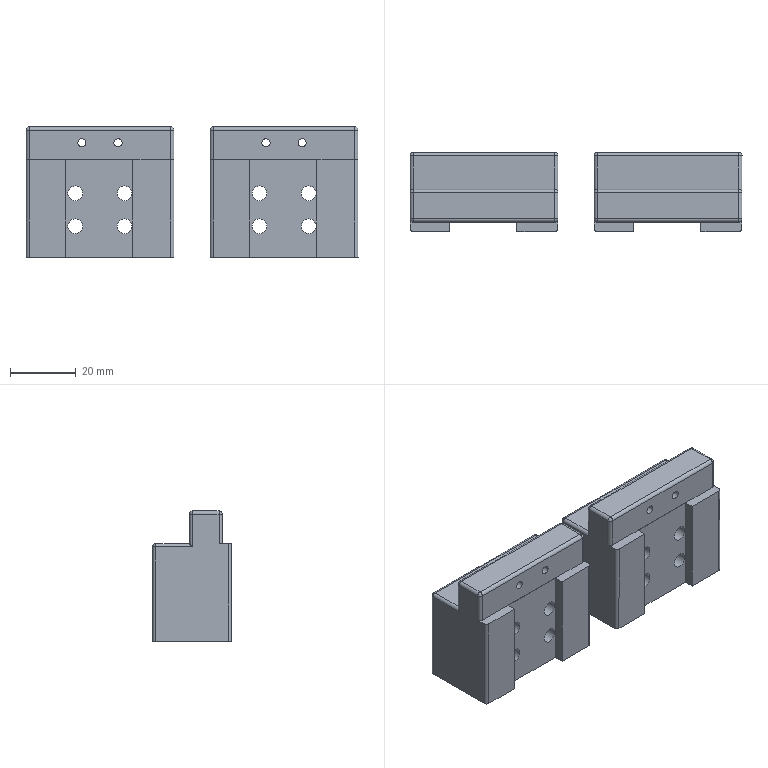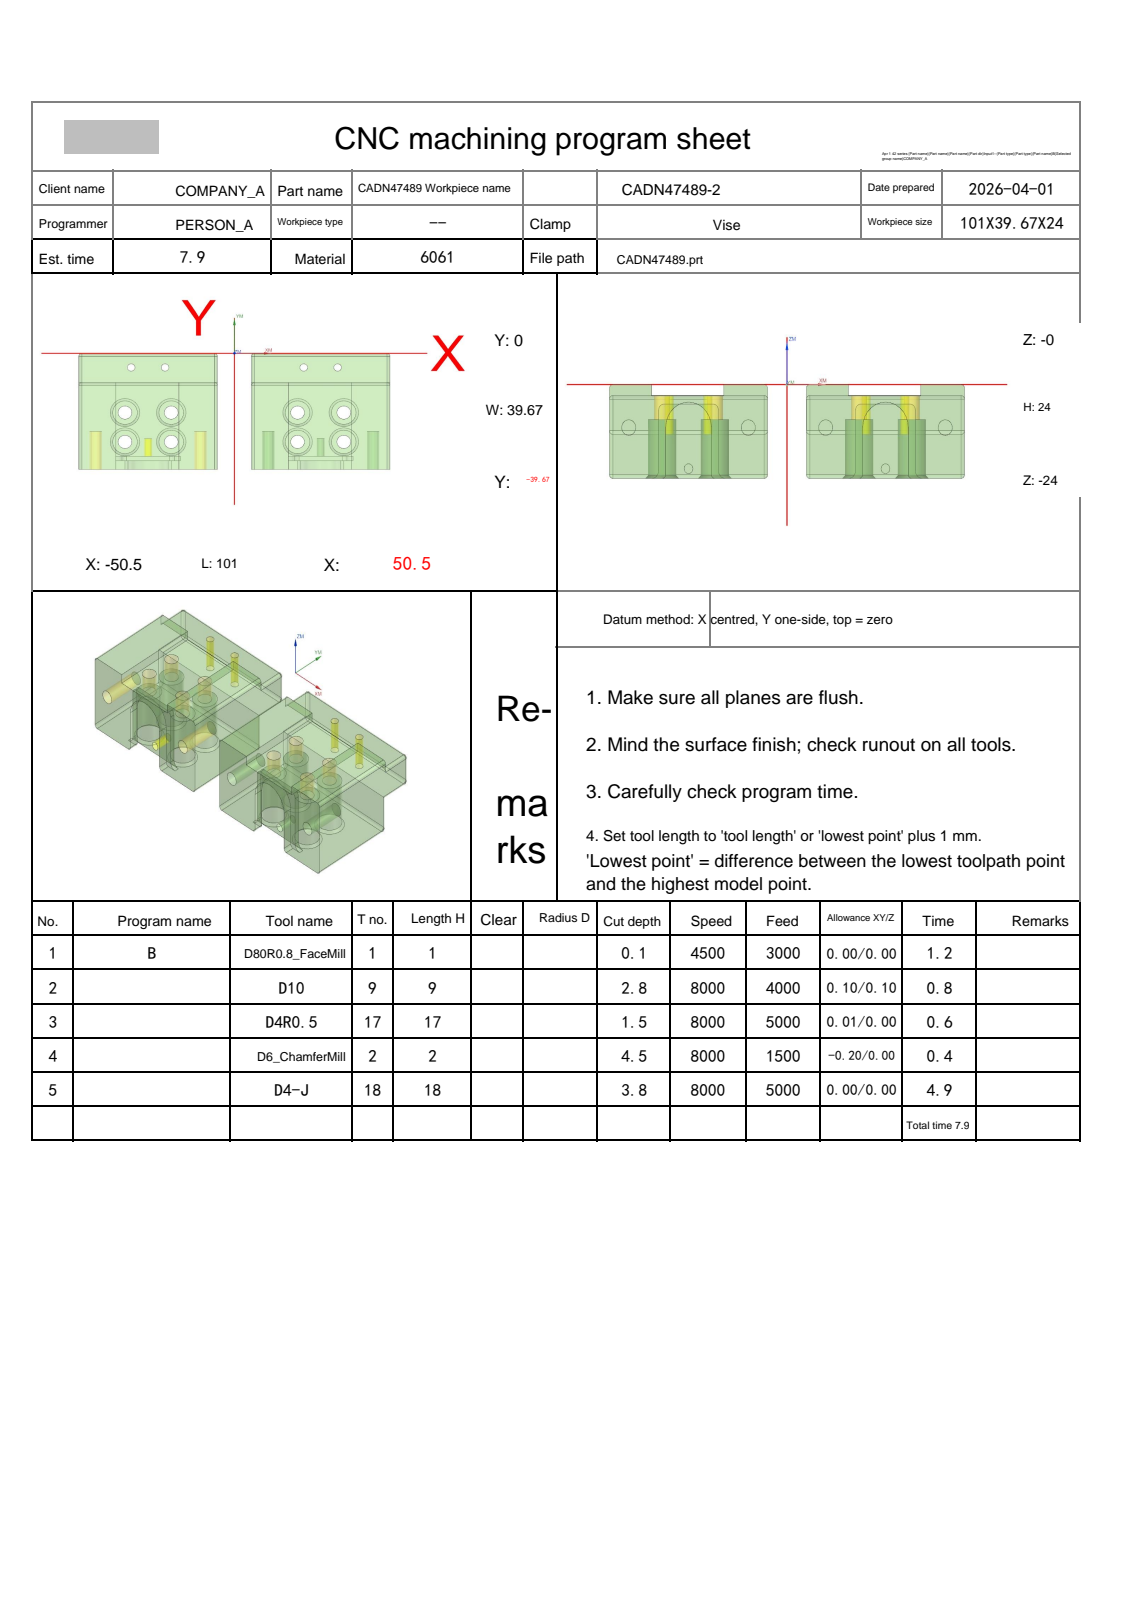NC program | NX | posted by the shop | part box 101.001 x 24.001 x 39.667 mm
Lines 1815 to 3048 of 5289:
N5 T18 M06
(D4-J  D=4. R=0. H=18 ce=0.40 di=0.00)
G00 G90 G54 X-35.75 Y-28.163 M03 S8000
G43 H18 Z10.5
M08
Z-1.701
G01 Y-29.709 Z-2.115 F800.
X-35.65 Y-29.663 Z-2.145
X-35.409 Y-29.651 Z-2.209
X-35.183 Y-29.733 Z-2.274
X-35.006 Y-29.897 Z-2.339
X-34.907 Y-30.117 Z-2.403
X-34.903 Y-30.227 Z-2.433
X-34.658 Y-30.327 Z-2.504
X-34.306 Y-30.537 Z-2.613
X-34.114 Y-30.682 Z-2.678
X-33.938 Y-30.856 Z-2.744
X-33.771 Y-31.039 Z-2.81
X-33.585 Y-31.321 Z-2.901
X-33.882 Y-31.506
G03 X-33.452 Y-30.251 I-1.617 J1.255
X-35.499 Y-28.204 I-2.047 J0.0
X-36.1 Y-28.294 I0.0 J-2.047
G01 Y-24.835
X-35.881 Y-24.856
X-35.728 Y-24.857
X-35.422 Y-24.829
X-35.114 Y-24.748
X-35.044 Y-24.728
X-34.809 Y-24.622
X-34.649 Y-24.543
X-34.48 Y-24.422
X-34.196 Y-24.174
X-34.142 Y-24.115
X-33.911 Y-23.808
X-33.809 Y-23.643
X-33.752 Y-23.502
X-33.639 Y-23.195
X-33.582 Y-22.888
X-33.571 Y-22.736
X-33.568 Y-22.582
X-33.584 Y-22.384
X-33.603 Y-22.276
X-33.672 Y-21.969
X-33.791 Y-21.663
X-33.882 Y-21.507
G03 X-33.452 Y-20.252 I-1.618 J1.255
X-35.5 Y-18.205 I-2.047 J0.0
X-36.1 Y-18.295 I0.0 J-2.047
G01 Y-12.402
X-20.4
Y-18.206
X-20.5 Y-18.203
G03 X-22.547 Y-20.25 I0.0 J-2.047
X-22.376 Y-21.07 I2.047 J0.0
G01 X-22.423 Y-21.121
X-22.617 Y-21.356
X-22.73 Y-21.538
X-22.801 Y-21.662
X-22.92 Y-21.969
X-22.996 Y-22.276
X-23.024 Y-22.582
X-23.007 Y-22.889
X-22.95 Y-23.195
X-22.841 Y-23.502
X-22.729 Y-23.728
X-22.68 Y-23.808
X-22.45 Y-24.115
X-22.281 Y-24.294
X-22.117 Y-24.418
X-21.81 Y-24.608
X-21.547 Y-24.728
X-21.198 Y-24.826
X-20.892 Y-24.854
X-20.585 Y-24.843
X-20.4 Y-24.827
Y-28.207
X-20.464 Y-28.205
X-20.539
G03 X-22.545 Y-30.251 I.04 J-2.046
X-22.375 Y-31.068 I2.046 J0.0
G01 X-22.544 Y-31.255
X-22.64 Y-31.394
X-22.744 Y-31.561
X-22.881 Y-31.868
X-22.977 Y-32.174
X-23.019 Y-32.481
Y-32.787
X-22.969 Y-33.093
X-22.88 Y-33.4
X-22.743 Y-33.707
X-22.542 Y-34.014
X-22.423 Y-34.144
X-22.247 Y-34.32
X-22.117 Y-34.418
X-21.81 Y-34.609
X-21.775 Y-34.626
X-21.504 Y-34.74
X-21.198 Y-34.826
X-20.892 Y-34.855
X-20.585 Y-34.844
X-20.4 Y-34.827
Y-39.67
X-20.393 Y-39.853
X-36.107 Y-39.854
X-36.1 Y-39.666
Y-34.835
X-35.881 Y-34.856
X-35.728 Y-34.857
X-35.422 Y-34.829
X-35.115 Y-34.748
X-34.962 Y-34.699
X-34.81 Y-34.623
X-34.502 Y-34.439
X-34.345 Y-34.32
X-34.196 Y-34.175
X-34.049 Y-34.013
X-33.89 Y-33.773
X-33.849 Y-33.707
X-33.712 Y-33.4
X-33.663 Y-33.246
X-33.638 Y-33.163
X-33.58 Y-33.1
X-31.568 Y-30.843
G03 X-31.469 Y-30.613 I-.299 J.266
X-31.452 Y-30.251 I-4.031 J.362
X-33.399 Y-26.792 I-4.047 J0.0
G02 X-33.59 Y-26.45 I.209 J.341
X-33.424 Y-26.126 I.4 J0.0
G01 X-33.237 Y-25.991
X-32.794 Y-25.606
X-32.6 Y-25.392
X-32.258 Y-24.937
X-32.022 Y-24.556
X-31.886 Y-24.225
X-31.704 Y-23.726
X-31.596 Y-23.147
X-31.572 Y-22.825
X-31.567 Y-22.52
X-31.598 Y-22.125
X-31.643 Y-21.879
X-31.672 Y-21.747
X-31.682 Y-21.661
X-31.661 Y-21.536
G03 X-31.452 Y-20.252 I-3.838 J1.284
X-33.863 Y-16.55 I-4.047 J0.0
G02 X-34.1 Y-16.186 I.163 J.365
G01 Y-14.801
G02 X-33.701 Y-14.402 I.4 J-.001
G01 X-22.799
G02 X-22.4 Y-14.801 I-.001 J-.4
G01 Y-16.445
G02 X-22.592 Y-16.786 I-.4 J.001
G03 X-24.547 Y-20.25 I2.092 J-3.464
X-24.537 Y-20.534 I4.047 J0.0
G01 X-24.536 Y-20.561
G02 X-24.589 Y-20.759 I-.4 J0.0
G01 X-24.611 Y-20.798
X-24.832 Y-21.366
X-24.974 Y-21.944
X-25.029 Y-22.545
X-24.997 Y-23.126
X-24.888 Y-23.717
X-24.686 Y-24.282
X-24.481 Y-24.698
X-24.334 Y-24.936
X-23.982 Y-25.405
X-23.622 Y-25.787
X-23.25 Y-26.069
X-22.879 Y-26.299
G02 X-22.691 Y-26.638 I-.212 J-.339
X-22.857 Y-26.963 I-.4 J0.0
G03 X-24.545 Y-30.251 I2.358 J-3.288
X-24.534 Y-30.549 I4.046 J0.0
G01 X-24.525 Y-30.615
X-24.536 Y-30.681
X-24.567 Y-30.74
X-24.755 Y-31.159
X-24.935 Y-31.736
X-25.019 Y-32.343
Y-32.95
X-24.923 Y-33.534
X-24.763 Y-34.091
X-24.503 Y-34.67
X-24.128 Y-35.243
X-23.869 Y-35.526
X-23.562 Y-35.833
X-23.251 Y-36.068
X-22.782 Y-36.36
X-22.622 Y-36.438
G02 X-22.4 Y-36.795 I-.178 J-.358
G01 Y-37.454
G02 X-22.799 Y-37.853 I-.4 J.001
G01 X-33.701 Y-37.854
G02 X-34.1 Y-37.455 I.001 J.4
G01 Y-36.75
G02 X-33.88 Y-36.394 I.4 J-.001
G01 X-33.846 Y-36.377
X-33.383 Y-36.1
X-33.039 Y-35.84
X-32.757 Y-35.565
X-32.467 Y-35.246
X-32.206 Y-34.853
X-32.078 Y-34.647
X-31.838 Y-34.11
X-31.664 Y-33.556
X-31.599 Y-33.156
X-31.573 Y-32.886
G02 X-31.446 Y-32.597 I.4 J-.004
G01 X-29.588 Y-30.862
G03 X-29.462 Y-30.593 I-.273 J.292
X-29.452 Y-30.251 I-6.037 J.342
X-30.663 Y-26.621 I-6.047 J0.0
G02 X-30.742 Y-26.382 I.321 J.239
X-30.663 Y-26.143 I.4 J0.0
G01 X-30.605 Y-26.067
X-30.234 Y-25.468
X-30.021 Y-24.948
X-29.769 Y-24.256
X-29.609 Y-23.406
X-29.573 Y-22.915
X-29.566 Y-22.457
X-29.612 Y-21.866
X-29.621 Y-21.816
X-29.637 Y-21.734
X-29.617 Y-21.653
G03 X-29.452 Y-20.252 I-5.883 J1.401
X-30.392 Y-17.015 I-6.047 J0.0
G02 X-30.453 Y-16.802 I.339 J.213
X-30.054 Y-16.402 I.4 J0.0
G01 X-25.946
G02 X-25.547 Y-16.802 I-.001 J-.4
X-25.609 Y-17.015 I-.4 J0.0
G03 X-26.547 Y-20.188 I5.109 J-3.236
G01 X-26.544 Y-20.26
X-26.573 Y-20.326
X-26.743 Y-20.763
X-26.952 Y-21.612
X-27.034 Y-22.508
X-26.987 Y-23.364
X-26.825 Y-24.239
X-26.531 Y-25.062
X-26.233 Y-25.668
X-25.988 Y-26.064
X-25.619 Y-26.556
G02 X-25.54 Y-26.795 I-.321 J-.239
X-25.602 Y-27.008 I-.4 J0.0
G03 X-26.544 Y-30.121 I5.103 J-3.243
G01 X-26.545 Y-30.183
X-26.544 Y-30.265
X-26.579 Y-30.339
X-26.629 Y-30.451
X-26.893 Y-31.298
X-27.019 Y-32.205
Y-33.113
X-26.878 Y-33.975
X-26.645 Y-34.781
X-26.416 Y-35.291
X-26.382 Y-35.453
G02 X-26.78 Y-35.853 I-.4 J0.0
G01 X-29.811
G02 X-30.21 Y-35.453 I.001 J.4
G01 X-30.176 Y-35.291
X-29.965 Y-34.82
X-29.713 Y-34.019
X-29.615 Y-33.413
X-29.573 Y-32.983
Y-32.775
X-29.566 Y-32.703
X-28.452 Y-26.7
G03 X-28.43 Y-26.461 I-1.287 J.238
G01 X-28.433 Y-26.378
X-28.442 Y-26.35
X-28.424 Y-26.326
X-28.395 Y-26.254
X-28.284 Y-26.18
X-28.177 Y-26.247
X-27.985 Y-26.638
X-27.862 Y-26.836
X-27.833 Y-26.882
X-27.829 Y-26.937
X-27.853 Y-26.986
X-27.999 Y-27.08
X-28.05 Y-27.072
X-28.095 Y-27.061
X-28.129 Y-27.029
X-28.145 Y-26.986
X-28.173 Y-26.923
Z-1.901
G00 Z8.5
X20.25 Y-28.16
Z-1.701
G01 Y-29.708 Z-2.116
X20.35 Y-29.662 Z-2.145
X20.539 Y-29.644 Z-2.196
X20.752 Y-29.697 Z-2.255
X20.971 Y-29.867 Z-2.329
X21.092 Y-30.116 Z-2.404
X21.097 Y-30.226 Z-2.433
X21.344 Y-30.328 Z-2.505
X21.694 Y-30.536 Z-2.614
X21.887 Y-30.682 Z-2.679
X22.062 Y-30.855 Z-2.745
X22.23 Y-31.039 Z-2.811
X22.414 Y-31.318 Z-2.901
X22.117 Y-31.504
G03 X22.547 Y-30.249 I-1.617 J1.255
X20.501 Y-28.203 I-2.047 J0.0
X19.9 Y-28.293 I0.0 J-2.047
G01 Y-24.834
X20.119 Y-24.855
X20.272 Y-24.856
X20.578 Y-24.828
X20.886 Y-24.747
X20.952 Y-24.728
X21.191 Y-24.622
X21.498 Y-24.438
X21.519 Y-24.422
X21.804 Y-24.173
X21.857 Y-24.115
X22.088 Y-23.808
X22.19 Y-23.643
X22.249 Y-23.502
X22.36 Y-23.195
X22.416 Y-22.897
X22.432 Y-22.582
X22.416 Y-22.383
X22.397 Y-22.276
X22.328 Y-21.969
X22.21 Y-21.663
X22.117 Y-21.505
G03 X22.547 Y-20.25 I-1.618 J1.255
X20.5 Y-18.202 I-2.047 J0.0
X19.9 Y-18.292 I0.0 J-2.047
G01 Y-12.401
X35.6
Y-18.205
X35.5 Y-18.202
G03 X33.453 Y-20.249 I0.0 J-2.047
X33.625 Y-21.069 I2.047 J0.0
G01 X33.577 Y-21.12
X33.382 Y-21.356
X33.27 Y-21.537
X33.198 Y-21.662
X33.079 Y-21.969
X33.004 Y-22.276
X32.976 Y-22.582
X32.993 Y-22.889
X33.05 Y-23.195
X33.159 Y-23.502
X33.271 Y-23.728
X33.32 Y-23.808
X33.552 Y-24.115
X33.576 Y-24.142
X33.883 Y-24.417
X34.19 Y-24.608
X34.456 Y-24.728
X34.802 Y-24.825
X35.108 Y-24.854
X35.415 Y-24.843
X35.6 Y-24.826
Y-28.207
X35.501 Y-28.204
G03 X33.455 Y-30.251 I0.0 J-2.046
X33.625 Y-31.068 I2.046 J0.0
G01 X33.455 Y-31.255
X33.359 Y-31.393
X33.256 Y-31.561
X33.119 Y-31.868
X33.023 Y-32.174
X32.981 Y-32.481
Y-32.787
X33.031 Y-33.093
X33.121 Y-33.401
X33.181 Y-33.557
X33.258 Y-33.706
X33.458 Y-34.014
X33.577 Y-34.143
X33.755 Y-34.32
X33.883 Y-34.416
X34.19 Y-34.608
X34.227 Y-34.626
X34.496 Y-34.74
X34.802 Y-34.825
X35.108 Y-34.853
X35.415 Y-34.843
X35.6 Y-34.827
Y-39.669
X35.607 Y-39.852
X19.893 Y-39.853
X19.9 Y-39.665
Y-34.834
X20.119 Y-34.855
X20.272 Y-34.856
X20.578 Y-34.828
X20.885 Y-34.747
X21.037 Y-34.698
X21.19 Y-34.622
X21.498 Y-34.438
X21.654 Y-34.32
X21.804 Y-34.174
X21.95 Y-34.013
X22.11 Y-33.772
X22.151 Y-33.707
X22.227 Y-33.557
X22.288 Y-33.401
X22.337 Y-33.246
X22.362 Y-33.164
X22.419 Y-33.1
X24.432 Y-30.838
G03 X24.531 Y-30.608 I-.299 J.266
X24.547 Y-30.249 I-4.031 J.359
X22.601 Y-26.791 I-4.047 J0.0
G02 X22.41 Y-26.449 I.209 J.341
X22.618 Y-26.098 I.4 J0.0
G01 X22.781 Y-25.975
X23.203 Y-25.607
X23.397 Y-25.395
X23.742 Y-24.936
X23.975 Y-24.558
X24.113 Y-24.228
X24.295 Y-23.725
X24.407 Y-23.132
X24.436 Y-22.554
X24.402 Y-22.124
X24.357 Y-21.878
X24.327 Y-21.745
X24.318 Y-21.659
X24.338 Y-21.533
G03 X24.547 Y-20.25 I-3.838 J1.283
X22.137 Y-16.548 I-4.047 J0.0
G02 X21.9 Y-16.184 I.163 J.365
G01 Y-14.8
G02 X22.299 Y-14.401 I.4 J-.001
G01 X33.201
G02 X33.6 Y-14.8 I-.001 J-.4
G01 Y-16.445
G02 X33.408 Y-16.785 I-.4 J.001
G03 X31.453 Y-20.249 I2.092 J-3.464
X31.463 Y-20.532 I4.047 J0.0
G01 X31.464 Y-20.559
G02 X31.411 Y-20.758 I-.4 J0.0
G01 X31.389 Y-20.797
X31.167 Y-21.368
X31.026 Y-21.946
X30.971 Y-22.545
X31.003 Y-23.128
X31.113 Y-23.717
X31.314 Y-24.281
X31.52 Y-24.7
X31.668 Y-24.939
X32.01 Y-25.394
X32.168 Y-25.566
X32.679 Y-26.024
X33.122 Y-26.299
G02 X33.309 Y-26.638 I-.212 J-.339
X33.143 Y-26.962 I-.4 J0.0
G03 X31.455 Y-30.251 I2.358 J-3.289
X31.466 Y-30.549 I4.046 J0.0
G01 X31.475 Y-30.614
X31.463 Y-30.68
X31.432 Y-30.739
X31.244 Y-31.161
X31.065 Y-31.738
X30.981 Y-32.343
Y-32.95
X31.077 Y-33.536
X31.224 Y-34.04
X31.353 Y-34.378
X31.528 Y-34.715
X31.872 Y-35.242
X32.132 Y-35.527
X32.441 Y-35.835
X32.75 Y-36.068
X33.213 Y-36.355
X33.38 Y-36.439
G02 X33.6 Y-36.795 I-.18 J-.357
G01 Y-37.453
G02 X33.201 Y-37.852 I-.4 J.001
G01 X22.299 Y-37.853
G02 X21.9 Y-37.454 I.001 J.4
G01 Y-36.749
G02 X22.121 Y-36.393 I.4 J-.001
G01 X22.152 Y-36.378
X22.618 Y-36.099
X22.961 Y-35.839
X23.242 Y-35.565
X23.531 Y-35.248
X23.795 Y-34.851
X23.895 Y-34.689
X24.054 Y-34.377
X24.176 Y-34.064
X24.336 Y-33.555
X24.401 Y-33.155
X24.427 Y-32.887
Y-32.884
G02 X24.554 Y-32.593 I.4 J-.001
G01 X26.411 Y-30.859
G03 X26.538 Y-30.59 I-.273 J.292
X26.547 Y-30.249 I-6.037 J.34
X25.337 Y-26.62 I-6.047 J0.0
G02 X25.258 Y-26.381 I.321 J.239
X25.337 Y-26.142 I.4 J0.0
G01 X25.396 Y-26.064
X25.761 Y-25.473
X25.977 Y-24.954
X26.231 Y-24.254
X26.398 Y-23.368
X26.44 Y-22.525
X26.388 Y-21.864
X26.379 Y-21.813
X26.362 Y-21.731
X26.383 Y-21.65
G03 X26.547 Y-20.25 I-5.883 J1.4
X25.609 Y-17.014 I-6.047 J0.0
G02 X25.547 Y-16.801 I.339 J.213
X25.946 Y-16.401 I.4 J0.0
G01 X30.054
G02 X30.453 Y-16.801 I-.001 J-.4
X30.391 Y-17.014 I-.4 J0.0
G03 X29.454 Y-20.186 I5.108 J-3.235
G01 X29.456 Y-20.258
X29.427 Y-20.324
X29.255 Y-20.766
X29.048 Y-21.615
X28.966 Y-22.508
X29.013 Y-23.368
X29.176 Y-24.239
X29.468 Y-25.061
X29.77 Y-25.673
X30.016 Y-26.069
X30.381 Y-26.554
G02 X30.46 Y-26.793 I-.321 J-.239
X30.398 Y-27.007 I-.4 J0.0
G03 X29.455 Y-30.182 I5.103 J-3.244
G01 X29.456 Y-30.264
X29.421 Y-30.338
X29.369 Y-30.454
X29.106 Y-31.301
X28.981 Y-32.205
Y-33.113
X29.123 Y-33.979
X29.327 Y-34.68
X29.526 Y-35.198
X29.563 Y-35.27
X29.607 Y-35.452
G02 X29.209 Y-35.852 I-.4 J0.0
G01 X26.199 Y-35.853
G02 X25.8 Y-35.453 I.001 J.4
G01 X25.843 Y-35.272
X25.881 Y-35.197
X26.064 Y-34.727
X26.287 Y-34.017
X26.385 Y-33.412
X26.427 Y-32.985
Y-32.772
X26.434 Y-32.7
X27.546 Y-26.7
G03 X27.568 Y-26.461 I-1.29 J.239
G01 X27.565 Y-26.375
X27.557 Y-26.346
X27.574 Y-26.321
X27.604 Y-26.251
X27.714 Y-26.177
X27.821 Y-26.244
X28.019 Y-26.645
X28.138 Y-26.835
X28.167 Y-26.881
X28.171 Y-26.936
X28.147 Y-26.985
X28.001 Y-27.079
X27.95 Y-27.071
X27.905 Y-27.06
X27.871 Y-27.029
X27.855 Y-26.985
X27.827 Y-26.923
Z-1.901
G00 Z10.5
X-48.954 Y-1.363
Z-1.284
G01 Z-2.784
Y-2.605
G03 X-49.754 Y-3.405 I0.0 J-.8
G01 Y-7.426
Y-7.565
X-49.748 Y-7.602
X-49.816
Y-3.405
X-49.814 Y-3.397
X-49.804 Y-3.375
X-49.798 Y-3.356
X-49.776 Y-3.355
X-49.769 Y-3.374
X-49.757 Y-3.396
X-49.754 Y-3.405
Y-3.605
Z-1.784
G00 Z8.5
X-50.435 Y-1.47
Z-1.284
G01 Z-2.784
Y-2.563
G03 X-49.635 Y-3.363 I.8 J0.0
G01 X-6.797
X-6.776 Y-3.362
X-6.777 Y-3.383
Y-7.426
Y-7.601
X-18.
G03 X-20.4 Y-10.001 I0.0 J-2.4
G01 Y-12.001
X-36.1 Y-12.002
Y-10.002
G03 X-38.5 Y-7.602 I-2.4 J0.0
G01 X-49.52
Y-5.602
Y-3.438
X-49.637 Y-3.423
X-49.657
X-49.655 Y-3.403
X-49.646 Y-3.406
X-49.581 Y-3.422
X-49.53 Y-3.465
X-49.506 Y-3.481
X-46.602 Y-5.302
G03 X-46.39 Y-5.363 I.212 J.339
G01 X-8.856
X-8.812 Y-5.366
X-8.779 Y-5.398
X-8.777 Y-5.443
Y-5.522
X-8.779 Y-5.566
X-8.812 Y-5.599
X-8.856 Y-5.601
X-18.
G03 X-22.385 Y-9.636 I0.0 J-4.4
G02 X-22.782 Y-10.001 I-.399 J.034
G01 X-33.718 Y-10.002
G02 X-34.115 Y-9.636 I.001 J.4
G01 X-34.121 Y-9.578
X-34.122 Y-9.544
G02 X-34.021 Y-9.293 I.36 J0.0
G01 X-32.642 Y-7.874
G03 X-32.53 Y-7.624 I-.287 J.279
G02 X-32.251 Y-7.363 I.279 J-.02
G01 X-24.249
G02 X-23.97 Y-7.643 I-.001 J-.28
G01 X-23.988 Y-7.741
X-24.016 Y-7.818
G02 X-24.278 Y-8.001 I-.263 J.097
G01 X-31.617 Y-8.002
X-31.672 Y-7.998
X-34.666 Y-7.584
G02 X-34.935 Y-7.422 I.055 J.396
G03 X-38.5 Y-5.602 I-3.565 J-2.579
G01 X-47.441
X-47.485 Y-5.6
X-47.518 Y-5.567
X-47.52 Y-5.522
Y-5.443
X-47.524 Y-5.41
X-47.498 Y-5.388
X-47.476 Y-5.361
X-47.441 Y-5.363
X-47.305
Z-1.784
G00 Z8.5
X5.412 Y-1.528
Z-1.284
G01 Z-2.784
Y-2.563
G03 X6.212 Y-3.363 I.8 J0.0
G01 X49.203
X49.224 Y-3.362
X49.223 Y-3.383
Y-7.6
X38.
G03 X35.6 Y-10. I0.0 J-2.4
G01 Y-12.
X19.9 Y-12.001
Y-10.001
G03 X17.5 Y-7.601 I-2.4 J0.0
G01 X6.48
Y-5.601
Y-3.437
X6.363 Y-3.422
X6.246 Y-3.407
Y-7.426
Y-7.601
X6.184
Y-4.367
X6.185 Y-4.333
X6.205 Y-4.102
G02 X6.604 Y-3.736 I.399 J-.034
X6.805 Y-3.791 I0.0 J-.4
G01 X9.492 Y-5.363
X47.144
X47.188 Y-5.365
X47.221 Y-5.398
X47.223 Y-5.442
Y-5.521
X47.221 Y-5.565
X47.188 Y-5.598
X47.144 Y-5.6
X38.
G03 X33.615 Y-9.635 I0.0 J-4.4
G02 X33.218 Y-10.001 I-.399 J.034
G01 X22.282
G02 X21.885 Y-9.635 I.001 J.4
G01 X21.879 Y-9.577
X21.878 Y-9.543
G02 X21.979 Y-9.292 I.36 J0.0
G01 X23.358 Y-7.873
G03 X23.47 Y-7.623 I-.287 J.279
G02 X23.749 Y-7.363 I.279 J-.02
G01 X31.751
G02 X32.03 Y-7.643 I-.001 J-.28
G01 X32.012 Y-7.741
X31.984 Y-7.817
G02 X31.722 Y-8.001 I-.263 J.097
G01 X24.383
X24.329 Y-7.997
X21.334 Y-7.583
G02 X21.065 Y-7.422 I.055 J.396
G03 X17.5 Y-5.601 I-3.565 J-2.579
G01 X8.56
X8.515 Y-5.599
X8.482 Y-5.566
X8.48 Y-5.521
Y-5.442
X8.476 Y-5.41
X8.5 Y-5.39
X8.523 Y-5.361
X8.56 Y-5.363
X8.692
Z-1.784
G00 Z8.5
X-35.75 Y-28.163
Z-1.7
G01 Y-29.709 Z-2.115
X-35.65 Y-29.663 Z-2.144
X-35.409 Y-29.651 Z-2.209
X-35.183 Y-29.733 Z-2.273
X-35.006 Y-29.897 Z-2.338
X-34.907 Y-30.117 Z-2.402
X-34.903 Y-30.227 Z-2.432
X-34.658 Y-30.327 Z-2.503
X-34.306 Y-30.537 Z-2.612
X-34.114 Y-30.682 Z-2.677
X-33.938 Y-30.856 Z-2.743
X-33.771 Y-31.039 Z-2.81
X-33.585 Y-31.321 Z-2.9
X-33.882 Y-31.506
G03 X-33.452 Y-30.251 I-1.617 J1.255
X-35.499 Y-28.204 I-2.047 J0.0
X-36.1 Y-28.294 I0.0 J-2.047
G01 Y-24.835
X-35.881 Y-24.856
X-35.728 Y-24.857
X-35.422 Y-24.829
X-35.114 Y-24.748
X-35.044 Y-24.728
X-34.809 Y-24.622
X-34.649 Y-24.543
X-34.48 Y-24.422
X-34.196 Y-24.174
X-34.142 Y-24.115
X-33.911 Y-23.808
X-33.809 Y-23.643
X-33.752 Y-23.502
X-33.639 Y-23.195
X-33.582 Y-22.888
X-33.571 Y-22.736
X-33.568 Y-22.582
X-33.584 Y-22.384
X-33.603 Y-22.276
X-33.672 Y-21.969
X-33.791 Y-21.663
X-33.882 Y-21.507
G03 X-33.452 Y-20.252 I-1.618 J1.255
X-35.5 Y-18.205 I-2.047 J0.0
X-36.1 Y-18.295 I0.0 J-2.047
G01 Y-12.402
X-20.4
Y-18.206
X-20.5 Y-18.203
G03 X-22.547 Y-20.25 I0.0 J-2.047
X-22.376 Y-21.07 I2.047 J0.0
G01 X-22.423 Y-21.121
X-22.617 Y-21.356
X-22.73 Y-21.538
X-22.801 Y-21.662
X-22.92 Y-21.969
X-22.996 Y-22.276
X-23.024 Y-22.582
X-23.007 Y-22.889
X-22.95 Y-23.195
X-22.841 Y-23.502
X-22.729 Y-23.728
X-22.68 Y-23.808
X-22.45 Y-24.115
X-22.281 Y-24.294
X-22.117 Y-24.418
X-21.81 Y-24.608
X-21.547 Y-24.728
X-21.198 Y-24.826
X-20.892 Y-24.854
X-20.585 Y-24.843
X-20.4 Y-24.827
Y-28.207
X-20.464 Y-28.205
X-20.539
G03 X-22.545 Y-30.251 I.04 J-2.046
X-22.375 Y-31.068 I2.046 J0.0
G01 X-22.544 Y-31.255
X-22.64 Y-31.394
X-22.744 Y-31.561
X-22.881 Y-31.868
X-22.977 Y-32.174
X-23.019 Y-32.481
Y-32.787
X-22.969 Y-33.093
X-22.88 Y-33.4
X-22.743 Y-33.707
X-22.542 Y-34.014
X-22.423 Y-34.144
X-22.247 Y-34.32
X-22.117 Y-34.418
X-21.81 Y-34.609
X-21.775 Y-34.626
X-21.504 Y-34.74
X-21.198 Y-34.826
X-20.892 Y-34.855
X-20.585 Y-34.844
X-20.4 Y-34.827
Y-39.67
X-20.393 Y-39.853
X-36.107 Y-39.854
X-36.1 Y-39.666
Y-34.835
X-35.881 Y-34.856
X-35.728 Y-34.857
X-35.422 Y-34.829
X-35.115 Y-34.748
X-34.962 Y-34.699
X-34.81 Y-34.623
X-34.502 Y-34.439
X-34.345 Y-34.32
X-34.196 Y-34.175
X-34.049 Y-34.013
X-33.89 Y-33.773
X-33.849 Y-33.707
X-33.712 Y-33.4
X-33.663 Y-33.246
X-33.638 Y-33.163
X-33.58 Y-33.1
X-31.568 Y-30.843
G03 X-31.469 Y-30.613 I-.299 J.266
X-31.452 Y-30.251 I-4.031 J.362
X-33.399 Y-26.792 I-4.047 J0.0
G02 X-33.59 Y-26.45 I.209 J.341
X-33.424 Y-26.126 I.4 J0.0
G01 X-33.237 Y-25.991
X-32.794 Y-25.606
X-32.6 Y-25.392
X-32.258 Y-24.937
X-32.022 Y-24.556
X-31.886 Y-24.225
X-31.704 Y-23.726
X-31.596 Y-23.147
X-31.572 Y-22.825
X-31.567 Y-22.52
X-31.598 Y-22.125
X-31.643 Y-21.879
X-31.672 Y-21.747
X-31.682 Y-21.661
X-31.661 Y-21.536
G03 X-31.452 Y-20.252 I-3.838 J1.284
X-33.863 Y-16.55 I-4.047 J0.0
G02 X-34.1 Y-16.186 I.163 J.365
G01 Y-14.801
G02 X-33.701 Y-14.402 I.4 J-.001
G01 X-22.799
G02 X-22.4 Y-14.801 I-.001 J-.4
G01 Y-16.445
G02 X-22.592 Y-16.786 I-.4 J.001
G03 X-24.547 Y-20.25 I2.092 J-3.464
X-24.537 Y-20.534 I4.047 J0.0
G01 X-24.536 Y-20.561
G02 X-24.589 Y-20.759 I-.4 J0.0
G01 X-24.611 Y-20.798
X-24.832 Y-21.366
X-24.974 Y-21.944
X-25.029 Y-22.545
X-24.997 Y-23.126
X-24.888 Y-23.717
X-24.686 Y-24.282
X-24.481 Y-24.698
X-24.334 Y-24.936
X-23.982 Y-25.405
X-23.622 Y-25.787
X-23.25 Y-26.069
X-22.879 Y-26.299
G02 X-22.691 Y-26.638 I-.212 J-.339
X-22.857 Y-26.963 I-.4 J0.0
G03 X-24.545 Y-30.251 I2.358 J-3.288
X-24.534 Y-30.549 I4.046 J0.0
G01 X-24.525 Y-30.615
X-24.536 Y-30.681
X-24.567 Y-30.74
X-24.755 Y-31.159
X-24.935 Y-31.736
X-25.019 Y-32.343
Y-32.95
X-24.923 Y-33.534
X-24.763 Y-34.091
X-24.503 Y-34.67
X-24.128 Y-35.243
X-23.869 Y-35.526
X-23.562 Y-35.833
X-23.251 Y-36.068
X-22.782 Y-36.36
X-22.622 Y-36.438
G02 X-22.4 Y-36.795 I-.178 J-.358
G01 Y-37.454
G02 X-22.799 Y-37.853 I-.4 J.001
G01 X-33.701 Y-37.854
G02 X-34.1 Y-37.455 I.001 J.4
G01 Y-36.75
G02 X-33.88 Y-36.394 I.4 J-.001
G01 X-33.846 Y-36.377
X-33.383 Y-36.1
X-33.039 Y-35.84
X-32.757 Y-35.565
X-32.467 Y-35.246
X-32.206 Y-34.853
X-32.078 Y-34.647
X-31.838 Y-34.11
X-31.664 Y-33.556
X-31.599 Y-33.156
X-31.573 Y-32.886
G02 X-31.446 Y-32.597 I.4 J-.004
G01 X-29.588 Y-30.862
G03 X-29.462 Y-30.593 I-.273 J.292
X-29.452 Y-30.251 I-6.037 J.342
X-30.663 Y-26.621 I-6.047 J0.0
G02 X-30.742 Y-26.382 I.321 J.239
X-30.663 Y-26.143 I.4 J0.0
G01 X-30.605 Y-26.067
X-30.234 Y-25.468
X-30.021 Y-24.948
X-29.769 Y-24.256
X-29.609 Y-23.406
X-29.573 Y-22.915
X-29.566 Y-22.457
X-29.612 Y-21.866
X-29.621 Y-21.816
X-29.637 Y-21.734
X-29.617 Y-21.653
G03 X-29.452 Y-20.252 I-5.883 J1.401
X-30.392 Y-17.015 I-6.047 J0.0
G02 X-30.453 Y-16.802 I.339 J.213
X-30.054 Y-16.402 I.4 J0.0
G01 X-25.946
G02 X-25.547 Y-16.802 I-.001 J-.4
X-25.609 Y-17.015 I-.4 J0.0
G03 X-26.547 Y-20.188 I5.109 J-3.236
G01 X-26.544 Y-20.26
X-26.573 Y-20.326
X-26.743 Y-20.763
X-26.952 Y-21.612
X-27.034 Y-22.508
X-26.987 Y-23.364
X-26.825 Y-24.239
X-26.531 Y-25.062
X-26.233 Y-25.668
X-25.988 Y-26.064
X-25.619 Y-26.556
G02 X-25.54 Y-26.795 I-.321 J-.239
X-25.602 Y-27.008 I-.4 J0.0
G03 X-26.544 Y-30.121 I5.103 J-3.243
G01 X-26.545 Y-30.183
X-26.544 Y-30.265
X-26.579 Y-30.339
X-26.629 Y-30.451
X-26.893 Y-31.298
X-27.019 Y-32.205
Y-33.113
X-26.878 Y-33.975
X-26.645 Y-34.781
X-26.416 Y-35.291
X-26.382 Y-35.453
G02 X-26.78 Y-35.853 I-.4 J0.0
G01 X-29.811
G02 X-30.21 Y-35.453 I.001 J.4
G01 X-30.176 Y-35.291
X-29.965 Y-34.82
X-29.713 Y-34.019
X-29.615 Y-33.413
X-29.573 Y-32.983
Y-32.775
X-29.566 Y-32.703
X-28.452 Y-26.7
G03 X-28.43 Y-26.461 I-1.287 J.238
G01 X-28.433 Y-26.378
X-28.442 Y-26.35
X-28.424 Y-26.326
X-28.395 Y-26.254
X-28.284 Y-26.18
X-28.177 Y-26.247
X-27.985 Y-26.638
X-27.862 Y-26.836
X-27.833 Y-26.882
X-27.829 Y-26.937
X-27.853 Y-26.986
X-27.999 Y-27.08
X-28.05 Y-27.072
X-28.095 Y-27.061
X-28.129 Y-27.029
X-28.145 Y-26.986
X-28.173 Y-26.923
Z-1.9
G00 Z8.5
X20.25 Y-28.16
Z-1.7
G01 Y-29.708 Z-2.115
X20.35 Y-29.662 Z-2.144
X20.539 Y-29.644 Z-2.195
X20.752 Y-29.697 Z-2.254
X20.971 Y-29.867 Z-2.328
X21.092 Y-30.116 Z-2.403
X21.097 Y-30.226 Z-2.432
X21.344 Y-30.328 Z-2.504
X21.694 Y-30.536 Z-2.613
X21.887 Y-30.682 Z-2.678
X22.062 Y-30.855 Z-2.744
X22.23 Y-31.039 Z-2.811
X22.414 Y-31.318 Z-2.9
X22.117 Y-31.504
G03 X22.547 Y-30.249 I-1.617 J1.255
X20.501 Y-28.203 I-2.047 J0.0
X19.9 Y-28.293 I0.0 J-2.047
G01 Y-24.834
X20.119 Y-24.855
X20.272 Y-24.856
X20.578 Y-24.828
X20.886 Y-24.747
X20.952 Y-24.728
X21.191 Y-24.622
X21.498 Y-24.438
X21.519 Y-24.422
X21.804 Y-24.173
X21.857 Y-24.115
X22.088 Y-23.808
X22.19 Y-23.643
X22.249 Y-23.502
X22.36 Y-23.195
X22.416 Y-22.897
X22.432 Y-22.582
X22.416 Y-22.383
X22.397 Y-22.276
X22.328 Y-21.969
X22.21 Y-21.663
X22.117 Y-21.505
G03 X22.547 Y-20.25 I-1.618 J1.255
X20.5 Y-18.202 I-2.047 J0.0
X19.9 Y-18.292 I0.0 J-2.047
G01 Y-12.401
X35.6
Y-18.205
X35.5 Y-18.202
G03 X33.453 Y-20.249 I0.0 J-2.047
X33.625 Y-21.069 I2.047 J0.0
G01 X33.577 Y-21.12
X33.382 Y-21.356
X33.27 Y-21.537
X33.198 Y-21.662
X33.079 Y-21.969
X33.004 Y-22.276
X32.976 Y-22.582
X32.993 Y-22.889
X33.05 Y-23.195
X33.159 Y-23.502
X33.271 Y-23.728
X33.32 Y-23.808
X33.552 Y-24.115
X33.576 Y-24.142
X33.883 Y-24.417
X34.19 Y-24.608
X34.456 Y-24.728
X34.802 Y-24.825
X35.108 Y-24.854
X35.415 Y-24.843
X35.6 Y-24.826
Y-28.207
X35.501 Y-28.204
G03 X33.455 Y-30.251 I0.0 J-2.046
X33.625 Y-31.068 I2.046 J0.0
G01 X33.455 Y-31.255
X33.359 Y-31.393
X33.256 Y-31.561
X33.119 Y-31.868
X33.023 Y-32.174
X32.981 Y-32.481
Y-32.787
X33.031 Y-33.093
X33.121 Y-33.401
X33.181 Y-33.557
X33.258 Y-33.706
X33.458 Y-34.014
X33.577 Y-34.143
X33.755 Y-34.32
X33.883 Y-34.416
X34.19 Y-34.608
X34.227 Y-34.626
X34.496 Y-34.74
X34.802 Y-34.825
X35.108 Y-34.853
X35.415 Y-34.843
X35.6 Y-34.827
Y-37.877
Y-39.669
X35.607 Y-39.852
X19.893 Y-39.853
X19.9 Y-39.665
Y-39.62
Y-34.834
X20.119 Y-34.855
X20.272 Y-34.856
X20.578 Y-34.828
X20.885 Y-34.747
X21.037 Y-34.698
X21.19 Y-34.622
X21.498 Y-34.438
X21.654 Y-34.32
X21.804 Y-34.174
X21.95 Y-34.013
X22.11 Y-33.772
X22.151 Y-33.707
X22.227 Y-33.557
X22.288 Y-33.401
X22.337 Y-33.246
X22.362 Y-33.164
X22.419 Y-33.1
X24.432 Y-30.838
G03 X24.531 Y-30.608 I-.299 J.266
X24.547 Y-30.249 I-4.031 J.359
X22.601 Y-26.791 I-4.047 J0.0
G02 X22.41 Y-26.449 I.209 J.341
X22.618 Y-26.098 I.4 J0.0
G01 X22.781 Y-25.975
X23.203 Y-25.607
X23.397 Y-25.395
X23.742 Y-24.936
X23.975 Y-24.558
X24.113 Y-24.228
X24.295 Y-23.725
X24.407 Y-23.132
X24.436 Y-22.554
X24.402 Y-22.124
X24.357 Y-21.878
X24.327 Y-21.745
X24.318 Y-21.659
X24.338 Y-21.533
G03 X24.547 Y-20.25 I-3.838 J1.284
X22.137 Y-16.548 I-4.047 J0.0
G02 X21.9 Y-16.184 I.163 J.365
G01 Y-14.8
G02 X22.299 Y-14.401 I.4 J-.001
G01 X33.201
G02 X33.6 Y-14.8 I-.001 J-.4
G01 Y-16.445
G02 X33.408 Y-16.785 I-.4 J.001
G03 X31.453 Y-20.249 I2.092 J-3.464
X31.463 Y-20.532 I4.047 J0.0
G01 X31.464 Y-20.559
G02 X31.411 Y-20.758 I-.4 J0.0
G01 X31.389 Y-20.797
X31.167 Y-21.368
X31.026 Y-21.946
X30.971 Y-22.545
X31.003 Y-23.128
X31.113 Y-23.717
X31.314 Y-24.281
X31.52 Y-24.7
X31.668 Y-24.939
X32.01 Y-25.394
X32.168 Y-25.566
X32.679 Y-26.024
X33.122 Y-26.299
G02 X33.309 Y-26.638 I-.212 J-.339
X33.143 Y-26.962 I-.4 J0.0
G03 X31.455 Y-30.251 I2.358 J-3.289
X31.466 Y-30.549 I4.046 J0.0
G01 X31.475 Y-30.614
X31.463 Y-30.68
X31.432 Y-30.739
X31.244 Y-31.161
X31.065 Y-31.738
X30.981 Y-32.343
Y-32.95
X31.077 Y-33.536
X31.224 Y-34.04
X31.353 Y-34.378
X31.528 Y-34.715
X31.872 Y-35.242
X32.132 Y-35.527
X32.441 Y-35.835
X32.75 Y-36.068
X33.213 Y-36.355
X33.38 Y-36.439
G02 X33.6 Y-36.795 I-.18 J-.357
G01 Y-37.453
G02 X33.201 Y-37.852 I-.4 J.001
G01 X22.299 Y-37.853
G02 X21.9 Y-37.454 I.001 J.4
G01 Y-36.749
G02 X22.121 Y-36.393 I.4 J-.001
G01 X22.152 Y-36.378
X22.618 Y-36.099
X22.961 Y-35.839
X23.242 Y-35.565
X23.531 Y-35.248
X23.795 Y-34.851
X23.895 Y-34.689
X24.054 Y-34.377
X24.176 Y-34.064
X24.336 Y-33.555
X24.401 Y-33.155
X24.427 Y-32.887
Y-32.884
G02 X24.554 Y-32.593 I.4 J-.001
G01 X26.411 Y-30.859
G03 X26.538 Y-30.59 I-.273 J.292